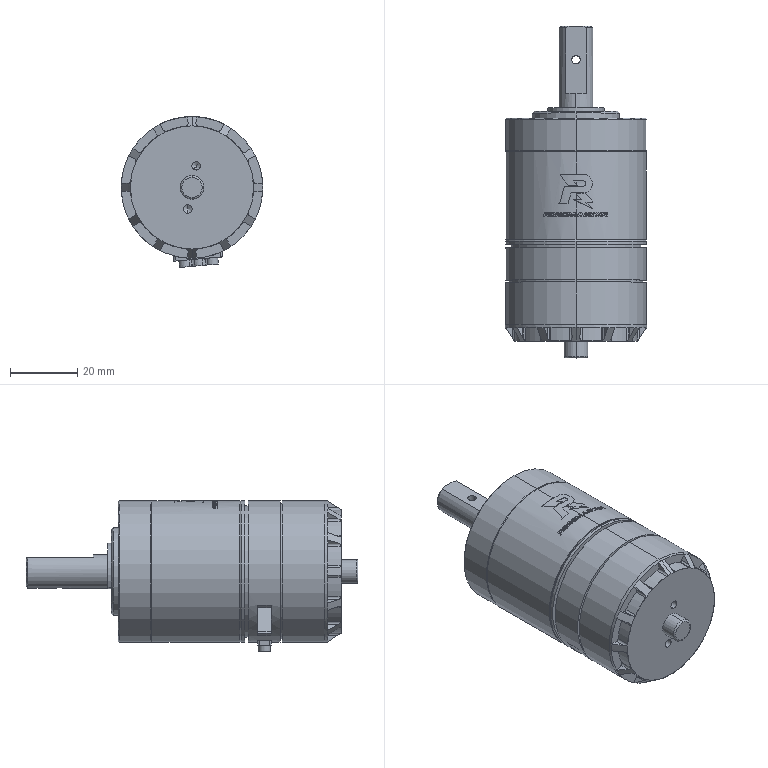Part | SolidWorks | features BaseBody 17 | 17 solids | 774 faces | box 42 x 98.4 x 44.727 mm | volume 85611 mm3 | cylinder 271 | plane 248 | spline 166 | torus 60 | cone 29 | commonest cylinder face diameters 1.4 x30 2 x24 20 x18 3 x16 42 x16 42.02 x14